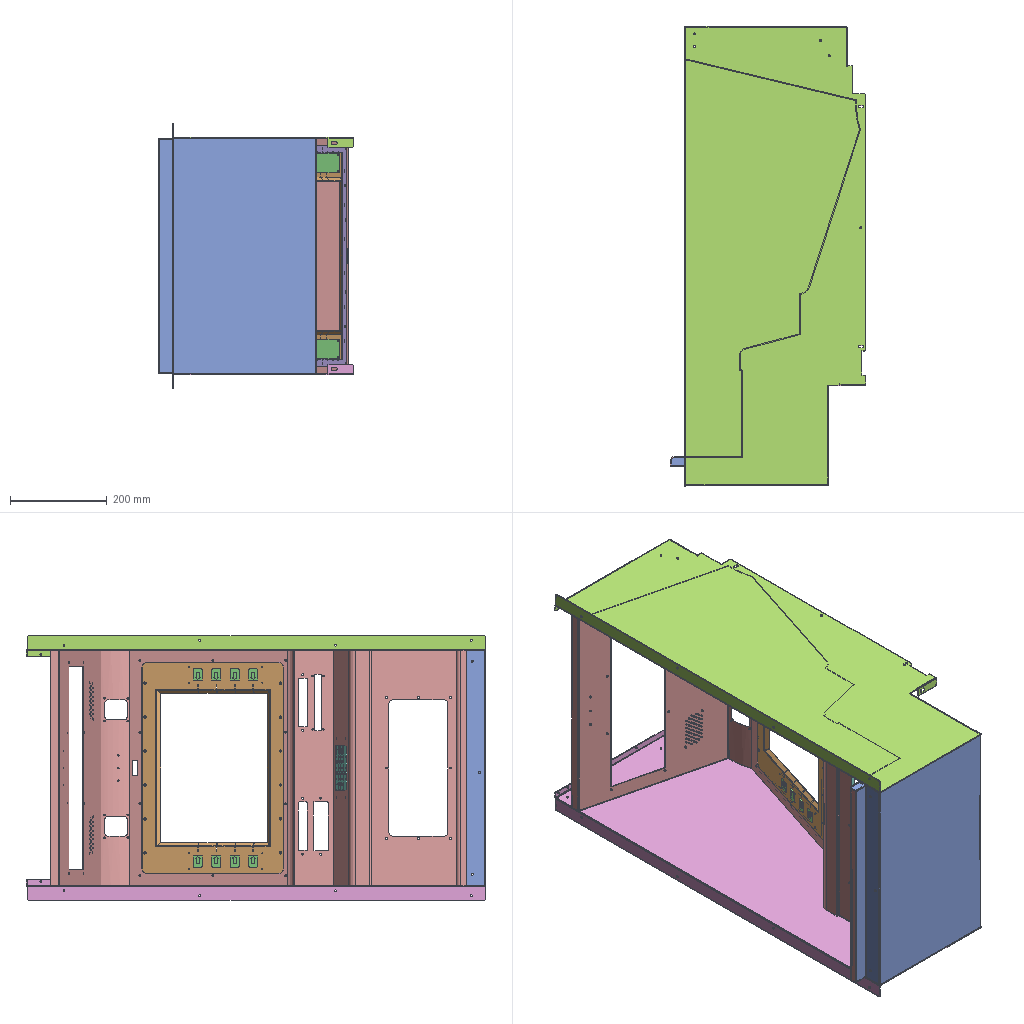Assembly | SolidWorks | 12 different items | 13 placed | box 403 x 948 x 545 mm
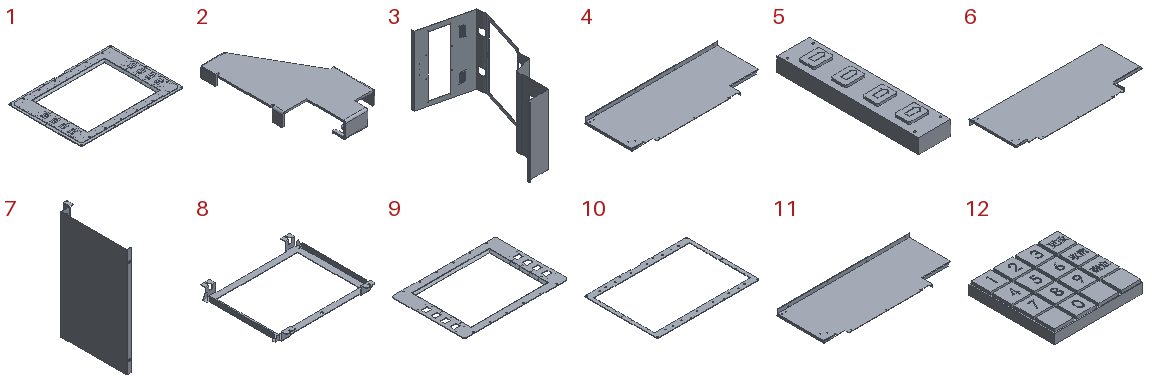Parts list (item | name | quantity | parent item | size | volume | features):
1 | (subassembly) | x1 | - | 455 x 325 x 21.5 mm | 462897 mm3 | -
2 | - | x1 | - | 75 x 136.5 x 18.5 mm | 16677 mm3 | features MirrorStock 1
3 | - | x1 | - | 392.354 x 858.638 x 485 mm | 871454 mm3 | features ICE 6, FlatPattern 1, Fold 1, SMBaseFlange 1, SheetMetal 1, UnFold 1
4 | - | x1 | - | 947.9 x 373 x 48 mm | 735400 mm3 | features MirrorStock 1
5 | - | x2 | in 1 | 40.5 x 178.5 x 21.5 mm | 138949 mm3 | features ICE 2, Extrusion 1, LPattern 1
6 | - | x1 | - | 947.9 x 373 x 48 mm | 735400 mm3 | features ICE 4, EdgeFlange 3, Fillet 1, FlatPattern 1, SMBaseFlange 1, SheetMetal 1
7 | - | x1 | - | 58 x 324.5 x 485 mm | 370922 mm3 | features ICE 2, EdgeFlange 1, Fillet 1, FlatPattern 1, SMBaseFlange 1, SheetMetal 1
8 | - | x1 | - | 354 x 314.5 x 31.5 mm | 59001 mm3 | features Jog 4, Chamfer 2, EdgeFlange 2, Fillet 1, FlatPattern 1, ICE 1, MirrorPattern 1, SMBaseFlange 1, SheetMetal 1
9 | - | x1 | in 1 | 435.6 x 305.6 x 9.192 mm | 120498 mm3 | features EdgeFlange 1, Fillet 1, FlatPattern 1, ICE 1, SMBaseFlange 1, SheetMetal 1
10 | - | x1 | in 1 | 455 x 325 x 2 mm | 64501 mm3 | features FlatPattern 1, SMBaseFlange 1, SheetMetal 1
11 | - | x1 | - | 947.9 x 373 x 48 mm | 735400 mm3 | features MirrorStock 1
12 | - | x1 | - | 92 x 88 x 13 mm | 100025 mm3 | features ICE 2, Extrusion 1
Mates (type | each side: item.copy, entity, surface, feature):
In the top assembly
Coincident | 3.1 face plane Base-Flange1 | 7.1 face plane Edge-Flange1 | 2 times
Concentric | 3.1 face cylinder Base bend12 | 7.1 face cylinder Fillet1
Coincident | 3.1 face plane Base-Flange1 | 6.1 face plane Base-Flange1
Coincident | 3.1 face plane Base-Flange1 | 6.1 face plane Edge-Flange4
Coincident | 7.1 face plane Base-Flange1 | 6.1 face plane Base-Flange1
DistanceDim | 12.1 face plane Boss-Extrude1 | 3.1 face plane Cut-Extrude6 | 2 times
DistanceDim | 12.1 face plane Boss-Extrude2 | 3.1 face plane Base-Flange1
Coincident | 3.1 face plane Base-Flange1 | 10.1 face plane Base-Flange1
Concentric | 3.1 face cylinder Cut-Extrude7 | 10.1 face cylinder Base-Flange1 | 2 times
In subassembly 1
Coincident | 9.1 face plane Base-Flange1 | 10.2 face plane Base-Flange1
Concentric | 9.1 face cylinder Base-Flange1 | 10.2 face cylinder Base-Flange1 | 2 times
Concentric | 9.1 face cylinder Base-Flange1 | 5.1 face cylinder Boss-Extrude1 | 2 times
Coincident | 9.1 face plane Base-Flange1 | 5.1 face plane Boss-Extrude1
Concentric | 9.1 face cylinder Base-Flange1 | 5.2 face cylinder Boss-Extrude1 | 2 times
Coincident | 9.1 face plane Base-Flange1 | 5.2 face plane Boss-Extrude1